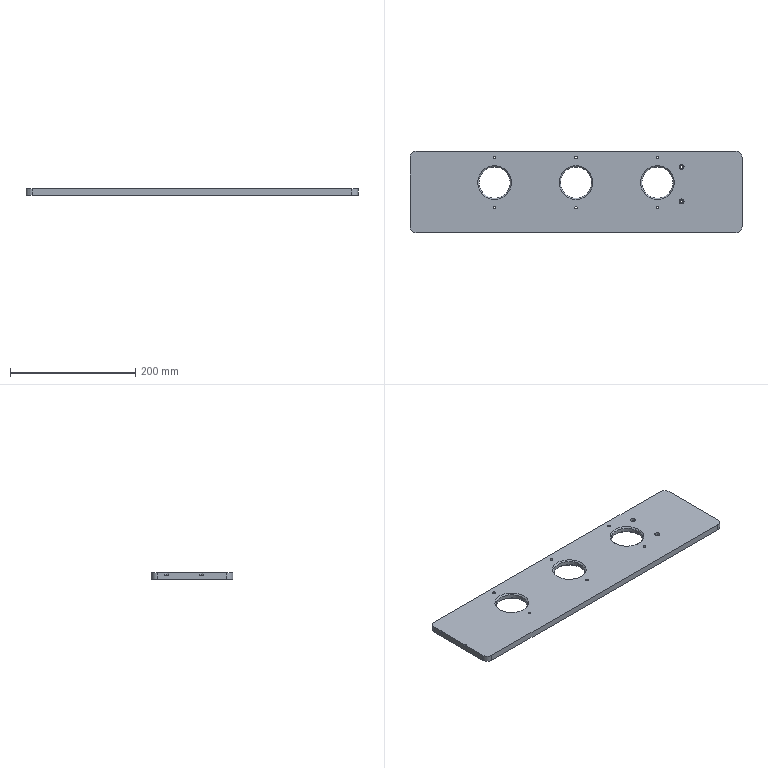Part | SolidWorks | features HoleWzd 2, Chamfer 1, Cut 1, Extrusion 1, Fillet 1, LPattern 1 | 1 solid | 56 faces | box 530 x 130 x 10 mm | volume 625792 mm3 | cylinder 34 | cone 12 | plane 10 | commonest cylinder face diameters 4.2 x12 8 x8 50 x6 4.5 x4 20 x4